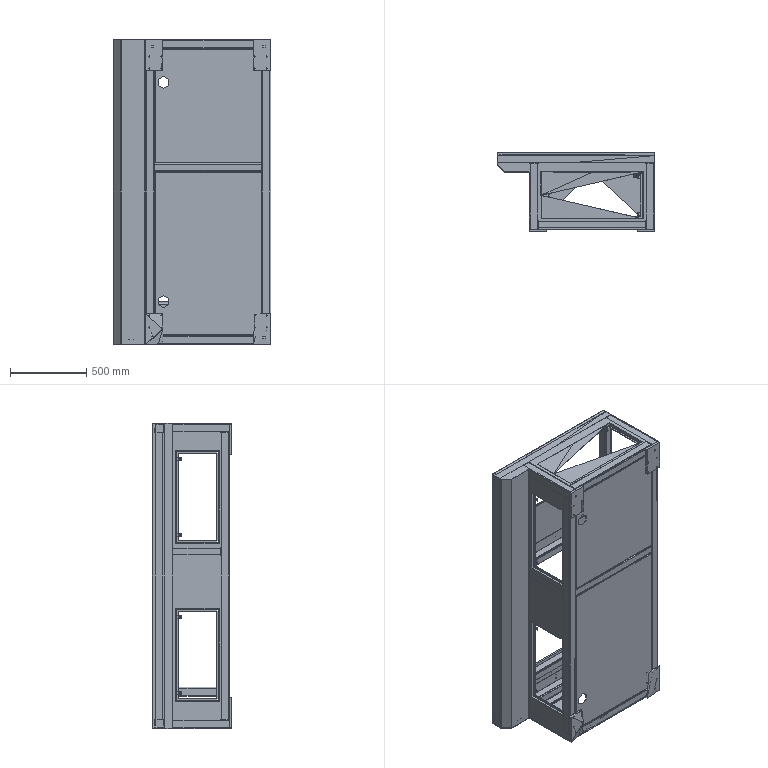Part | NX | features BREP 28 | 22 solids | 1266 faces | volume 10642783350498985553453068352448031461267152969419730003783267333393179734793694598415181955975914455040 mm3 | plane 629 | cylinder 514 | spline 84 | cone 39 | commonest cylinder face diameters 7 x79 8 x79 6.8 x77 16 x76 4 x57 8.5 x40